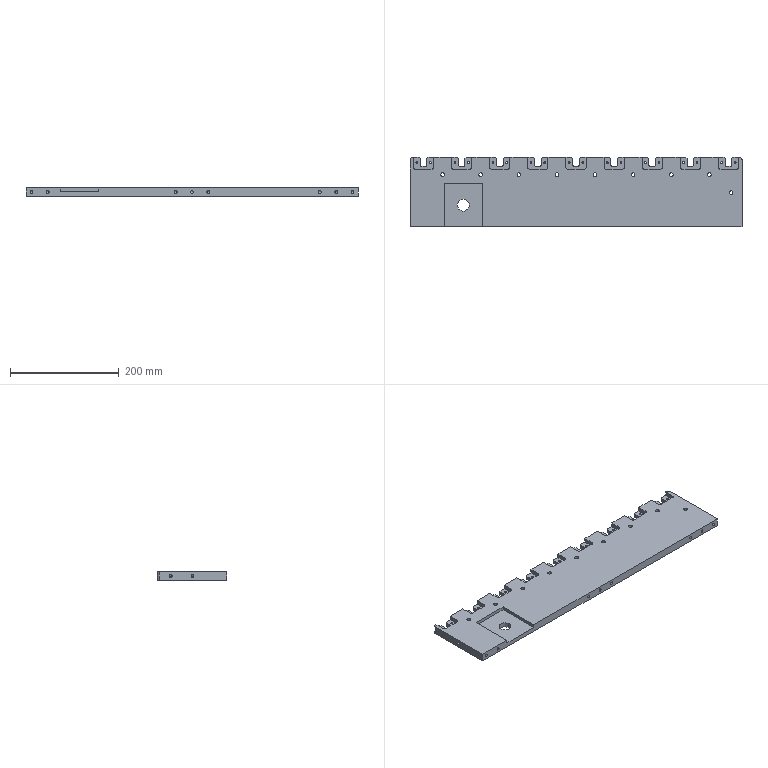Part | NX | 1 solid | 186 faces | box 610 x 128 x 15 mm | volume 1053411 mm3 | plane 100 | cylinder 76 | cone 10 | commonest cylinder face diameters 6 x36 3.3 x18 5 x10 6.8 x9 10 x2 22 x1